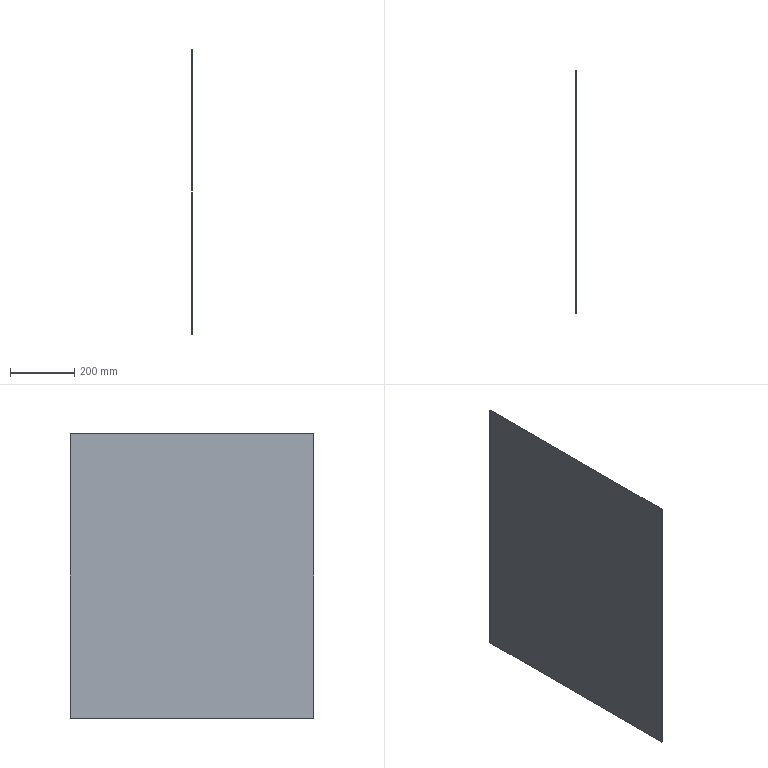Part | STEP file | Guide wheel mechanism revised.sldasm-Part-22 | 1 solid | 6 faces | box 1.2 x 760 x 890 mm | volume 811680 mm3 | plane 6
STEP:
#1=CARTESIAN_POINT('',(-485.,760.,445.));
#2=VERTEX_POINT('',#1);
#3=CARTESIAN_POINT('',(-485.,0.,445.));
#4=VERTEX_POINT('',#3);
#5=CARTESIAN_POINT('',(-485.,760.,445.));
#6=DIRECTION('',(0.,-1.,0.));
#7=VECTOR('',#6,1000.);
#8=LINE('',#5,#7);
#9=EDGE_CURVE('',#2,#4,#8,.T.);
#10=ORIENTED_EDGE('',*,*,#9,.F.);
#11=CARTESIAN_POINT('',(-486.2,760.,445.));
#12=VERTEX_POINT('',#11);
#13=CARTESIAN_POINT('',(-486.2,760.,445.));
#14=DIRECTION('',(1.,0.,0.));
#15=VECTOR('',#14,1000.);
#16=LINE('',#13,#15);
#17=EDGE_CURVE('',#12,#2,#16,.T.);
#18=ORIENTED_EDGE('',*,*,#17,.F.);
#19=CARTESIAN_POINT('',(-486.2,0.,445.));
#20=VERTEX_POINT('',#19);
#21=CARTESIAN_POINT('',(-486.2,760.,445.));
#22=DIRECTION('',(0.,-1.,0.));
#23=VECTOR('',#22,1000.);
#24=LINE('',#21,#23);
#25=EDGE_CURVE('',#12,#20,#24,.T.);
#26=ORIENTED_EDGE('',*,*,#25,.T.);
#27=CARTESIAN_POINT('',(-486.2,0.,445.));
#28=DIRECTION('',(1.,0.,0.));
#29=VECTOR('',#28,1000.);
#30=LINE('',#27,#29);
#31=EDGE_CURVE('',#20,#4,#30,.T.);
#32=ORIENTED_EDGE('',*,*,#31,.T.);
#33=EDGE_LOOP('',(#10,#18,#26,#32));
#34=FACE_OUTER_BOUND('',#33,.T.);
#35=CARTESIAN_POINT('',(-486.2,760.,445.));
#36=DIRECTION('',(0.,0.,1.));
#37=DIRECTION('',(0.,-1.,0.));
#38=AXIS2_PLACEMENT_3D('',#35,#36,#37);
#39=PLANE('',#38);
#40=ADVANCED_FACE('',(#34),#39,.T.);
#41=CARTESIAN_POINT('',(-485.,760.,-445.));
#42=VERTEX_POINT('',#41);
#43=CARTESIAN_POINT('',(-485.,760.,445.));
#44=DIRECTION('',(0.,0.,1.));
#45=VECTOR('',#44,1000.);
#46=LINE('',#43,#45);
#47=EDGE_CURVE('',#42,#2,#46,.T.);
#48=ORIENTED_EDGE('',*,*,#47,.F.);
#49=CARTESIAN_POINT('',(-486.2,760.,-445.));
#50=VERTEX_POINT('',#49);
#51=CARTESIAN_POINT('',(-486.2,760.,-445.));
#52=DIRECTION('',(1.,0.,0.));
#53=VECTOR('',#52,1000.);
#54=LINE('',#51,#53);
#55=EDGE_CURVE('',#50,#42,#54,.T.);
#56=ORIENTED_EDGE('',*,*,#55,.F.);
#57=CARTESIAN_POINT('',(-486.2,760.,445.));
#58=DIRECTION('',(0.,0.,1.));
#59=VECTOR('',#58,1000.);
#60=LINE('',#57,#59);
#61=EDGE_CURVE('',#50,#12,#60,.T.);
#62=ORIENTED_EDGE('',*,*,#61,.T.);
#63=ORIENTED_EDGE('',*,*,#17,.T.);
#64=EDGE_LOOP('',(#48,#56,#62,#63));
#65=FACE_OUTER_BOUND('',#64,.T.);
#66=CARTESIAN_POINT('',(-486.2,760.,445.));
#67=DIRECTION('',(0.,1.,0.));
#68=DIRECTION('',(0.,0.,1.));
#69=AXIS2_PLACEMENT_3D('',#66,#67,#68);
#70=PLANE('',#69);
#71=ADVANCED_FACE('',(#65),#70,.T.);
#72=CARTESIAN_POINT('',(-485.,0.,-445.));
#73=VERTEX_POINT('',#72);
#74=CARTESIAN_POINT('',(-485.,760.,-445.));
#75=DIRECTION('',(0.,1.,0.));
#76=VECTOR('',#75,1000.);
#77=LINE('',#74,#76);
#78=EDGE_CURVE('',#73,#42,#77,.T.);
#79=ORIENTED_EDGE('',*,*,#78,.F.);
#80=CARTESIAN_POINT('',(-486.2,0.,-445.));
#81=VERTEX_POINT('',#80);
#82=CARTESIAN_POINT('',(-486.2,0.,-445.));
#83=DIRECTION('',(1.,0.,0.));
#84=VECTOR('',#83,1000.);
#85=LINE('',#82,#84);
#86=EDGE_CURVE('',#81,#73,#85,.T.);
#87=ORIENTED_EDGE('',*,*,#86,.F.);
#88=CARTESIAN_POINT('',(-486.2,760.,-445.));
#89=DIRECTION('',(0.,1.,0.));
#90=VECTOR('',#89,1000.);
#91=LINE('',#88,#90);
#92=EDGE_CURVE('',#81,#50,#91,.T.);
#93=ORIENTED_EDGE('',*,*,#92,.T.);
#94=ORIENTED_EDGE('',*,*,#55,.T.);
#95=EDGE_LOOP('',(#79,#87,#93,#94));
#96=FACE_OUTER_BOUND('',#95,.T.);
#97=CARTESIAN_POINT('',(-486.2,760.,-445.));
#98=DIRECTION('',(0.,0.,-1.));
#99=DIRECTION('',(0.,1.,0.));
#100=AXIS2_PLACEMENT_3D('',#97,#98,#99);
#101=PLANE('',#100);
#102=ADVANCED_FACE('',(#96),#101,.T.);
#103=CARTESIAN_POINT('',(-485.,0.,445.));
#104=DIRECTION('',(0.,0.,-1.));
#105=VECTOR('',#104,1000.);
#106=LINE('',#103,#105);
#107=EDGE_CURVE('',#4,#73,#106,.T.);
#108=ORIENTED_EDGE('',*,*,#107,.F.);
#109=ORIENTED_EDGE('',*,*,#31,.F.);
#110=CARTESIAN_POINT('',(-486.2,0.,445.));
#111=DIRECTION('',(0.,0.,-1.));
#112=VECTOR('',#111,1000.);
#113=LINE('',#110,#112);
#114=EDGE_CURVE('',#20,#81,#113,.T.);
#115=ORIENTED_EDGE('',*,*,#114,.T.);
#116=ORIENTED_EDGE('',*,*,#86,.T.);
#117=EDGE_LOOP('',(#108,#109,#115,#116));
#118=FACE_OUTER_BOUND('',#117,.T.);
#119=CARTESIAN_POINT('',(-486.2,0.,445.));
#120=DIRECTION('',(0.,-1.,0.));
#121=DIRECTION('',(0.,0.,-1.));
#122=AXIS2_PLACEMENT_3D('',#119,#120,#121);
#123=PLANE('',#122);
#124=ADVANCED_FACE('',(#118),#123,.T.);
#125=ORIENTED_EDGE('',*,*,#25,.F.);
#126=ORIENTED_EDGE('',*,*,#61,.F.);
#127=ORIENTED_EDGE('',*,*,#92,.F.);
#128=ORIENTED_EDGE('',*,*,#114,.F.);
#129=EDGE_LOOP('',(#125,#126,#127,#128));
#130=FACE_OUTER_BOUND('',#129,.T.);
#131=CARTESIAN_POINT('',(-486.2,0.,0.));
#132=DIRECTION('',(1.,0.,0.));
#133=DIRECTION('',(0.,0.,-1.));
#134=AXIS2_PLACEMENT_3D('',#131,#132,#133);
#135=PLANE('',#134);
#136=ADVANCED_FACE('',(#130),#135,.F.);
#137=ORIENTED_EDGE('',*,*,#9,.T.);
#138=ORIENTED_EDGE('',*,*,#107,.T.);
#139=ORIENTED_EDGE('',*,*,#78,.T.);
#140=ORIENTED_EDGE('',*,*,#47,.T.);
#141=EDGE_LOOP('',(#137,#138,#139,#140));
#142=FACE_OUTER_BOUND('',#141,.T.);
#143=CARTESIAN_POINT('',(-485.,0.,0.));
#144=DIRECTION('',(1.,0.,0.));
#145=DIRECTION('',(0.,0.,-1.));
#146=AXIS2_PLACEMENT_3D('',#143,#144,#145);
#147=PLANE('',#146);
#148=ADVANCED_FACE('',(#142),#147,.T.);
#149=CLOSED_SHELL('',(#40,#71,#102,#124,#136,#148));
#150=MANIFOLD_SOLID_BREP('',#149);
#151=CARTESIAN_POINT('',(0.,0.,0.));
#152=DIRECTION('',(0.,0.,1.));
#153=DIRECTION('',(1.,0.,0.));
#154=AXIS2_PLACEMENT_3D('',#151,#152,#153);
#155=(LENGTH_UNIT()NAMED_UNIT(*)SI_UNIT(.MILLI.,.METRE.));
#156=UNCERTAINTY_MEASURE_WITH_UNIT(LENGTH_MEASURE(0.00001),#155,'','');
#157=(NAMED_UNIT(*)PLANE_ANGLE_UNIT()SI_UNIT($,.RADIAN.));
#158=(NAMED_UNIT(*)SI_UNIT($,.STERADIAN.)SOLID_ANGLE_UNIT());
#159=(GEOMETRIC_REPRESENTATION_CONTEXT(3)GLOBAL_UNCERTAINTY_ASSIGNED_CONTEXT((#156))GLOBAL_UNIT_ASSIGNED_CONTEXT((#155,#157,#158))REPRESENTATION_CONTEXT('',''));
#160=ADVANCED_BREP_SHAPE_REPRESENTATION('',(#150,#154),#159);